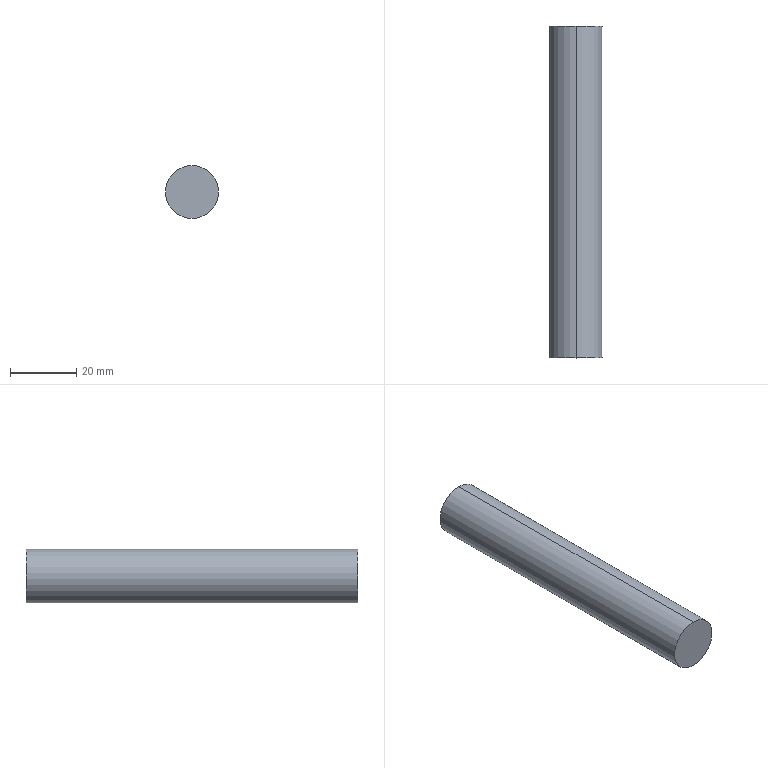Part | SolidWorks | features Extrusion 1 | 1 solid | 4 faces | box 16 x 100 x 16 mm | volume 20106 mm3 | cylinder 2 | plane 2 | commonest cylinder face diameters 16 x2
STEP:
#1=CARTESIAN_POINT('',(0.,100.,8.));
#2=VERTEX_POINT('',#1);
#3=CARTESIAN_POINT('',(0.,100.,-8.));
#4=VERTEX_POINT('',#3);
#5=CARTESIAN_POINT('',(0.,100.,0.));
#6=DIRECTION('',(0.,1.,0.));
#7=DIRECTION('',(0.,0.,1.));
#8=AXIS2_PLACEMENT_3D('',#5,#6,#7);
#9=CIRCLE('',#8,8.);
#10=EDGE_CURVE('',#2,#4,#9,.T.);
#11=ORIENTED_EDGE('',*,*,#10,.F.);
#12=CARTESIAN_POINT('',(0.,0.,8.));
#13=VERTEX_POINT('',#12);
#14=CARTESIAN_POINT('',(0.,100.,8.));
#15=DIRECTION('',(0.,-1.,0.));
#16=VECTOR('',#15,1000.);
#17=LINE('',#14,#16);
#18=EDGE_CURVE('',#2,#13,#17,.T.);
#19=ORIENTED_EDGE('',*,*,#18,.T.);
#20=CARTESIAN_POINT('',(0.,0.,-8.));
#21=VERTEX_POINT('',#20);
#22=CARTESIAN_POINT('',(0.,0.,0.));
#23=DIRECTION('',(0.,1.,0.));
#24=DIRECTION('',(0.,0.,1.));
#25=AXIS2_PLACEMENT_3D('',#22,#23,#24);
#26=CIRCLE('',#25,8.);
#27=EDGE_CURVE('',#13,#21,#26,.T.);
#28=ORIENTED_EDGE('',*,*,#27,.T.);
#29=CARTESIAN_POINT('',(0.,100.,-8.));
#30=DIRECTION('',(0.,-1.,0.));
#31=VECTOR('',#30,1000.);
#32=LINE('',#29,#31);
#33=EDGE_CURVE('',#4,#21,#32,.T.);
#34=ORIENTED_EDGE('',*,*,#33,.F.);
#35=EDGE_LOOP('',(#11,#19,#28,#34));
#36=FACE_OUTER_BOUND('',#35,.T.);
#37=CARTESIAN_POINT('',(0.,100.,0.));
#38=DIRECTION('',(0.,-1.,0.));
#39=DIRECTION('',(0.,0.,-1.));
#40=AXIS2_PLACEMENT_3D('',#37,#38,#39);
#41=CYLINDRICAL_SURFACE('',#40,8.);
#42=ADVANCED_FACE('',(#36),#41,.T.);
#43=ORIENTED_EDGE('',*,*,#18,.F.);
#44=CARTESIAN_POINT('',(0.,100.,0.));
#45=DIRECTION('',(0.,1.,0.));
#46=DIRECTION('',(0.,0.,1.));
#47=AXIS2_PLACEMENT_3D('',#44,#45,#46);
#48=CIRCLE('',#47,8.);
#49=EDGE_CURVE('',#4,#2,#48,.T.);
#50=ORIENTED_EDGE('',*,*,#49,.F.);
#51=ORIENTED_EDGE('',*,*,#33,.T.);
#52=CARTESIAN_POINT('',(0.,0.,0.));
#53=DIRECTION('',(0.,1.,0.));
#54=DIRECTION('',(0.,0.,1.));
#55=AXIS2_PLACEMENT_3D('',#52,#53,#54);
#56=CIRCLE('',#55,8.);
#57=EDGE_CURVE('',#21,#13,#56,.T.);
#58=ORIENTED_EDGE('',*,*,#57,.T.);
#59=EDGE_LOOP('',(#43,#50,#51,#58));
#60=FACE_OUTER_BOUND('',#59,.T.);
#61=CARTESIAN_POINT('',(0.,100.,0.));
#62=DIRECTION('',(0.,-1.,0.));
#63=DIRECTION('',(0.,0.,-1.));
#64=AXIS2_PLACEMENT_3D('',#61,#62,#63);
#65=CYLINDRICAL_SURFACE('',#64,8.);
#66=ADVANCED_FACE('',(#60),#65,.T.);
#67=ORIENTED_EDGE('',*,*,#49,.T.);
#68=ORIENTED_EDGE('',*,*,#10,.T.);
#69=EDGE_LOOP('',(#67,#68));
#70=FACE_OUTER_BOUND('',#69,.T.);
#71=CARTESIAN_POINT('',(0.,100.,0.));
#72=DIRECTION('',(0.,1.,0.));
#73=DIRECTION('',(0.,0.,1.));
#74=AXIS2_PLACEMENT_3D('',#71,#72,#73);
#75=PLANE('',#74);
#76=ADVANCED_FACE('',(#70),#75,.T.);
#77=ORIENTED_EDGE('',*,*,#57,.F.);
#78=ORIENTED_EDGE('',*,*,#27,.F.);
#79=EDGE_LOOP('',(#77,#78));
#80=FACE_OUTER_BOUND('',#79,.T.);
#81=CARTESIAN_POINT('',(0.,0.,0.));
#82=DIRECTION('',(0.,1.,0.));
#83=DIRECTION('',(0.,0.,1.));
#84=AXIS2_PLACEMENT_3D('',#81,#82,#83);
#85=PLANE('',#84);
#86=ADVANCED_FACE('',(#80),#85,.F.);
#87=CLOSED_SHELL('',(#42,#66,#76,#86));
#88=MANIFOLD_SOLID_BREP('',#87);
#89=CARTESIAN_POINT('',(0.,0.,0.));
#90=DIRECTION('',(0.,0.,1.));
#91=DIRECTION('',(1.,0.,0.));
#92=AXIS2_PLACEMENT_3D('',#89,#90,#91);
#93=(LENGTH_UNIT()NAMED_UNIT(*)SI_UNIT(.MILLI.,.METRE.));
#94=UNCERTAINTY_MEASURE_WITH_UNIT(LENGTH_MEASURE(0.00001),#93,'','');
#95=(NAMED_UNIT(*)PLANE_ANGLE_UNIT()SI_UNIT($,.RADIAN.));
#96=(NAMED_UNIT(*)SI_UNIT($,.STERADIAN.)SOLID_ANGLE_UNIT());
#97=(GEOMETRIC_REPRESENTATION_CONTEXT(3)GLOBAL_UNCERTAINTY_ASSIGNED_CONTEXT((#94))GLOBAL_UNIT_ASSIGNED_CONTEXT((#93,#95,#96))REPRESENTATION_CONTEXT('',''));
#98=ADVANCED_BREP_SHAPE_REPRESENTATION('',(#88,#92),#97);